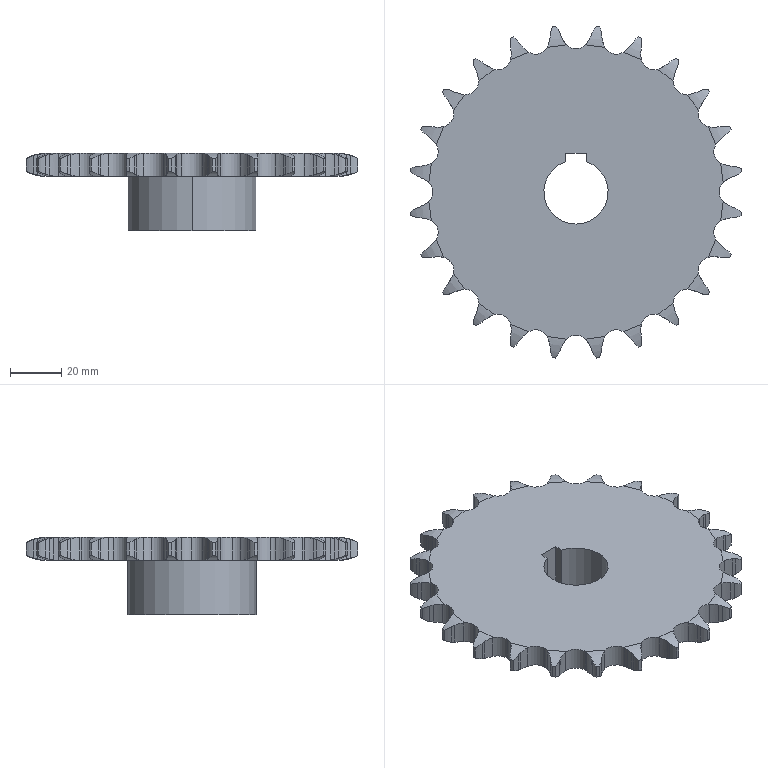Part | SolidWorks | features BaseBody 1 | 1 solid | 261 faces | box 129.139 x 129.139 x 30 mm | volume 122850 mm3 | cylinder 159 | plane 54 | spline 48 | commonest cylinder face diameters 16.697 x50 26.518 x50 10.262 x31 130.108 x24 25 x2 50 x2